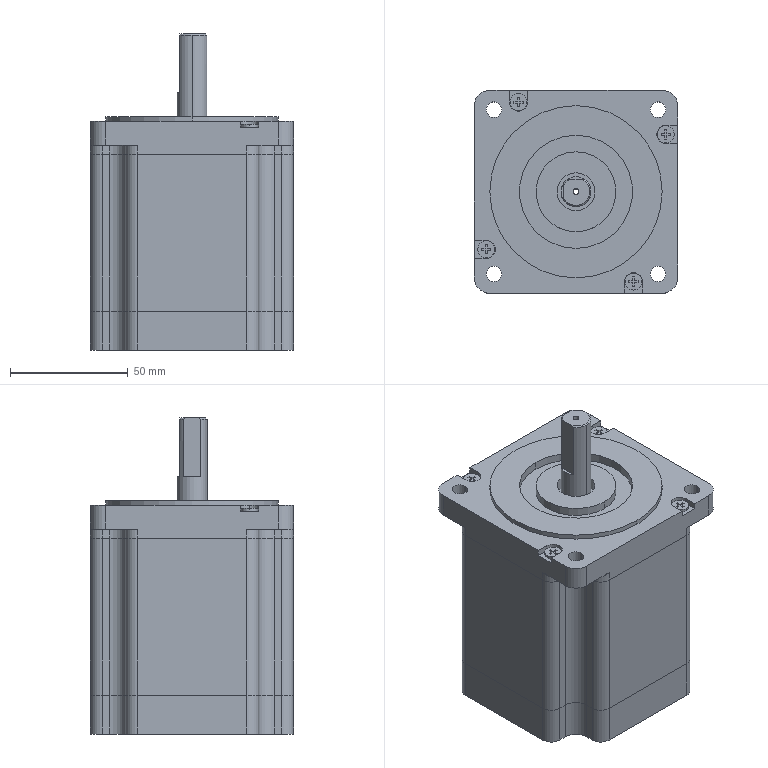Part | SolidWorks | features BaseBody 9 | 9 solids | 307 faces | box 86.106 x 86.131 x 134.112 mm | volume 651811 mm3 | plane 143 | cylinder 132 | cone 20 | spline 12 | commonest cylinder face diameters 4.166 x42 10.16 x25 13.005 x12 6.604 x8 7.178 x8 2.54 x6